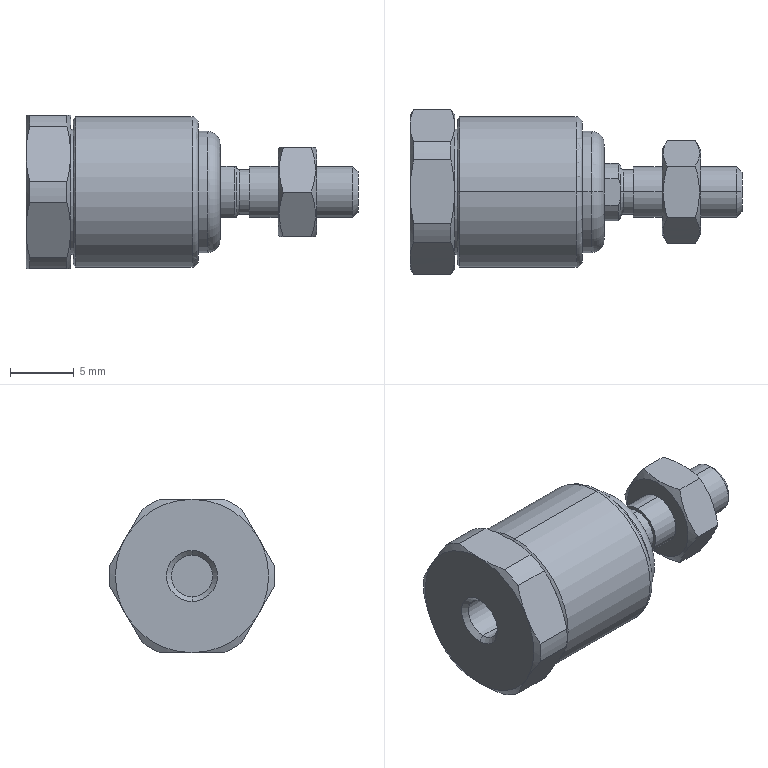Part | STEP file | F-M4X070F^Take-up clamp assembly | 1 solid | 83 faces | box 26 x 13 x 12 mm | volume 1801 mm3 | plane 27 | cone 26 | cylinder 22 | torus 8 | commonest cylinder face diameters 13 x6 4 x4 3.242 x2 3.5 x2 4.5 x2 9.5 x2